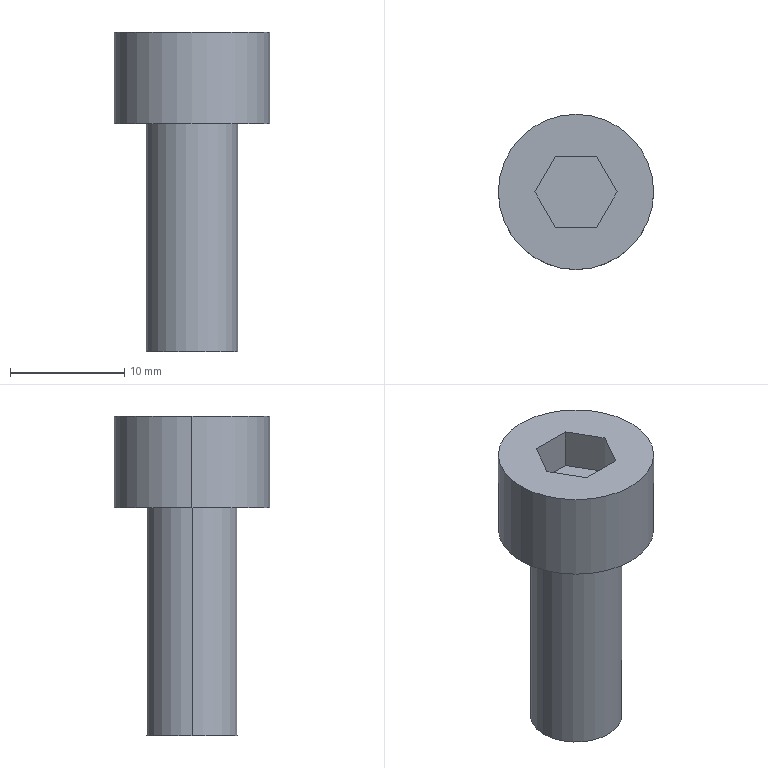Part | SolidWorks | features BaseBody 1 | 1 solid | 14 faces | box 13.6 x 13.6 x 28 mm | volume 2046 mm3 | plane 10 | cylinder 4 | commonest cylinder face diameters 8 x2 13.6 x2
STEP:
#1=CARTESIAN_POINT('',(4.,0.,-20.));
#2=VERTEX_POINT('',#1);
#3=CARTESIAN_POINT('',(-4.,0.,-20.));
#4=VERTEX_POINT('',#3);
#5=CARTESIAN_POINT('',(0.,0.,-20.));
#6=DIRECTION('',(0.,0.,1.));
#7=DIRECTION('',(1.,0.,0.));
#8=AXIS2_PLACEMENT_3D('',#5,#6,#7);
#9=CIRCLE('',#8,4.);
#10=EDGE_CURVE('',#2,#4,#9,.T.);
#11=ORIENTED_EDGE('',*,*,#10,.T.);
#12=CARTESIAN_POINT('',(-4.,0.,0.));
#13=VERTEX_POINT('',#12);
#14=CARTESIAN_POINT('',(-4.,0.,-20.));
#15=DIRECTION('',(0.,0.,1.));
#16=VECTOR('',#15,1000.);
#17=LINE('',#14,#16);
#18=EDGE_CURVE('',#4,#13,#17,.T.);
#19=ORIENTED_EDGE('',*,*,#18,.T.);
#20=CARTESIAN_POINT('',(4.,0.,0.));
#21=VERTEX_POINT('',#20);
#22=CARTESIAN_POINT('',(0.,0.,0.));
#23=DIRECTION('',(0.,0.,-1.));
#24=DIRECTION('',(1.,0.,0.));
#25=AXIS2_PLACEMENT_3D('',#22,#23,#24);
#26=CIRCLE('',#25,4.);
#27=EDGE_CURVE('',#13,#21,#26,.T.);
#28=ORIENTED_EDGE('',*,*,#27,.T.);
#29=CARTESIAN_POINT('',(4.,0.,-20.));
#30=DIRECTION('',(0.,0.,1.));
#31=VECTOR('',#30,1000.);
#32=LINE('',#29,#31);
#33=EDGE_CURVE('',#2,#21,#32,.T.);
#34=ORIENTED_EDGE('',*,*,#33,.F.);
#35=EDGE_LOOP('',(#11,#19,#28,#34));
#36=FACE_OUTER_BOUND('',#35,.T.);
#37=CARTESIAN_POINT('',(0.,0.,-20.));
#38=DIRECTION('',(0.,0.,1.));
#39=DIRECTION('',(1.,0.,0.));
#40=AXIS2_PLACEMENT_3D('',#37,#38,#39);
#41=CYLINDRICAL_SURFACE('',#40,4.);
#42=ADVANCED_FACE('',(#36),#41,.T.);
#43=CARTESIAN_POINT('',(6.8,0.,0.));
#44=VERTEX_POINT('',#43);
#45=CARTESIAN_POINT('',(-6.8,0.,0.));
#46=VERTEX_POINT('',#45);
#47=CARTESIAN_POINT('',(0.,0.,0.));
#48=DIRECTION('',(0.,0.,1.));
#49=DIRECTION('',(1.,0.,0.));
#50=AXIS2_PLACEMENT_3D('',#47,#48,#49);
#51=CIRCLE('',#50,6.8);
#52=EDGE_CURVE('',#44,#46,#51,.T.);
#53=ORIENTED_EDGE('',*,*,#52,.T.);
#54=CARTESIAN_POINT('',(-6.8,0.,8.));
#55=VERTEX_POINT('',#54);
#56=CARTESIAN_POINT('',(-6.8,0.,0.));
#57=DIRECTION('',(0.,0.,1.));
#58=VECTOR('',#57,1000.);
#59=LINE('',#56,#58);
#60=EDGE_CURVE('',#46,#55,#59,.T.);
#61=ORIENTED_EDGE('',*,*,#60,.T.);
#62=CARTESIAN_POINT('',(6.8,0.,8.));
#63=VERTEX_POINT('',#62);
#64=CARTESIAN_POINT('',(0.,0.,8.));
#65=DIRECTION('',(0.,0.,-1.));
#66=DIRECTION('',(1.,0.,0.));
#67=AXIS2_PLACEMENT_3D('',#64,#65,#66);
#68=CIRCLE('',#67,6.8);
#69=EDGE_CURVE('',#55,#63,#68,.T.);
#70=ORIENTED_EDGE('',*,*,#69,.T.);
#71=CARTESIAN_POINT('',(6.8,0.,0.));
#72=DIRECTION('',(0.,0.,1.));
#73=VECTOR('',#72,1000.);
#74=LINE('',#71,#73);
#75=EDGE_CURVE('',#44,#63,#74,.T.);
#76=ORIENTED_EDGE('',*,*,#75,.F.);
#77=EDGE_LOOP('',(#53,#61,#70,#76));
#78=FACE_OUTER_BOUND('',#77,.T.);
#79=CARTESIAN_POINT('',(0.,0.,0.));
#80=DIRECTION('',(0.,0.,1.));
#81=DIRECTION('',(1.,0.,0.));
#82=AXIS2_PLACEMENT_3D('',#79,#80,#81);
#83=CYLINDRICAL_SURFACE('',#82,6.8);
#84=ADVANCED_FACE('',(#78),#83,.T.);
#85=ORIENTED_EDGE('',*,*,#18,.F.);
#86=CARTESIAN_POINT('',(0.,0.,-20.));
#87=DIRECTION('',(0.,0.,1.));
#88=DIRECTION('',(1.,0.,0.));
#89=AXIS2_PLACEMENT_3D('',#86,#87,#88);
#90=CIRCLE('',#89,4.);
#91=EDGE_CURVE('',#4,#2,#90,.T.);
#92=ORIENTED_EDGE('',*,*,#91,.T.);
#93=ORIENTED_EDGE('',*,*,#33,.T.);
#94=CARTESIAN_POINT('',(0.,0.,0.));
#95=DIRECTION('',(0.,0.,-1.));
#96=DIRECTION('',(1.,0.,0.));
#97=AXIS2_PLACEMENT_3D('',#94,#95,#96);
#98=CIRCLE('',#97,4.);
#99=EDGE_CURVE('',#21,#13,#98,.T.);
#100=ORIENTED_EDGE('',*,*,#99,.T.);
#101=EDGE_LOOP('',(#85,#92,#93,#100));
#102=FACE_OUTER_BOUND('',#101,.T.);
#103=CARTESIAN_POINT('',(0.,0.,-20.));
#104=DIRECTION('',(0.,0.,1.));
#105=DIRECTION('',(1.,0.,0.));
#106=AXIS2_PLACEMENT_3D('',#103,#104,#105);
#107=CYLINDRICAL_SURFACE('',#106,4.);
#108=ADVANCED_FACE('',(#102),#107,.T.);
#109=ORIENTED_EDGE('',*,*,#10,.F.);
#110=ORIENTED_EDGE('',*,*,#91,.F.);
#111=EDGE_LOOP('',(#109,#110));
#112=FACE_OUTER_BOUND('',#111,.T.);
#113=CARTESIAN_POINT('',(0.,0.,-20.));
#114=DIRECTION('',(0.,0.,1.));
#115=DIRECTION('',(1.,0.,0.));
#116=AXIS2_PLACEMENT_3D('',#113,#114,#115);
#117=PLANE('',#116);
#118=ADVANCED_FACE('',(#112),#117,.F.);
#119=ORIENTED_EDGE('',*,*,#99,.F.);
#120=ORIENTED_EDGE('',*,*,#27,.F.);
#121=EDGE_LOOP('',(#119,#120));
#122=FACE_BOUND('',#121,.T.);
#123=ORIENTED_EDGE('',*,*,#52,.F.);
#124=CARTESIAN_POINT('',(0.,0.,0.));
#125=DIRECTION('',(0.,0.,1.));
#126=DIRECTION('',(1.,0.,0.));
#127=AXIS2_PLACEMENT_3D('',#124,#125,#126);
#128=CIRCLE('',#127,6.8);
#129=EDGE_CURVE('',#46,#44,#128,.T.);
#130=ORIENTED_EDGE('',*,*,#129,.F.);
#131=EDGE_LOOP('',(#123,#130));
#132=FACE_OUTER_BOUND('',#131,.T.);
#133=CARTESIAN_POINT('',(0.,0.,0.));
#134=DIRECTION('',(0.,0.,1.));
#135=DIRECTION('',(1.,0.,0.));
#136=AXIS2_PLACEMENT_3D('',#133,#134,#135);
#137=PLANE('',#136);
#138=ADVANCED_FACE('',(#122,#132),#137,.F.);
#139=ORIENTED_EDGE('',*,*,#60,.F.);
#140=ORIENTED_EDGE('',*,*,#129,.T.);
#141=ORIENTED_EDGE('',*,*,#75,.T.);
#142=CARTESIAN_POINT('',(0.,0.,8.));
#143=DIRECTION('',(0.,0.,-1.));
#144=DIRECTION('',(1.,0.,0.));
#145=AXIS2_PLACEMENT_3D('',#142,#143,#144);
#146=CIRCLE('',#145,6.8);
#147=EDGE_CURVE('',#63,#55,#146,.T.);
#148=ORIENTED_EDGE('',*,*,#147,.T.);
#149=EDGE_LOOP('',(#139,#140,#141,#148));
#150=FACE_OUTER_BOUND('',#149,.T.);
#151=CARTESIAN_POINT('',(0.,0.,0.));
#152=DIRECTION('',(0.,0.,1.));
#153=DIRECTION('',(1.,0.,0.));
#154=AXIS2_PLACEMENT_3D('',#151,#152,#153);
#155=CYLINDRICAL_SURFACE('',#154,6.8);
#156=ADVANCED_FACE('',(#150),#155,.T.);
#157=CARTESIAN_POINT('',(-1.8,-3.118,8.));
#158=VERTEX_POINT('',#157);
#159=CARTESIAN_POINT('',(-3.6,0.,8.));
#160=VERTEX_POINT('',#159);
#161=CARTESIAN_POINT('',(-1.8,-3.118,8.));
#162=DIRECTION('',(-0.5,0.866,0.));
#163=VECTOR('',#162,1000.);
#164=LINE('',#161,#163);
#165=EDGE_CURVE('',#158,#160,#164,.T.);
#166=ORIENTED_EDGE('',*,*,#165,.T.);
#167=CARTESIAN_POINT('',(-1.8,3.118,8.));
#168=VERTEX_POINT('',#167);
#169=CARTESIAN_POINT('',(-3.6,0.,8.));
#170=DIRECTION('',(0.5,0.866,0.));
#171=VECTOR('',#170,1000.);
#172=LINE('',#169,#171);
#173=EDGE_CURVE('',#160,#168,#172,.T.);
#174=ORIENTED_EDGE('',*,*,#173,.T.);
#175=CARTESIAN_POINT('',(1.8,3.118,8.));
#176=VERTEX_POINT('',#175);
#177=CARTESIAN_POINT('',(0.,3.118,8.));
#178=DIRECTION('',(1.,0.,0.));
#179=VECTOR('',#178,1000.);
#180=LINE('',#177,#179);
#181=EDGE_CURVE('',#168,#176,#180,.T.);
#182=ORIENTED_EDGE('',*,*,#181,.T.);
#183=CARTESIAN_POINT('',(3.6,0.,8.));
#184=VERTEX_POINT('',#183);
#185=CARTESIAN_POINT('',(1.8,3.118,8.));
#186=DIRECTION('',(0.5,-0.866,0.));
#187=VECTOR('',#186,1000.);
#188=LINE('',#185,#187);
#189=EDGE_CURVE('',#176,#184,#188,.T.);
#190=ORIENTED_EDGE('',*,*,#189,.T.);
#191=CARTESIAN_POINT('',(1.8,-3.118,8.));
#192=VERTEX_POINT('',#191);
#193=CARTESIAN_POINT('',(3.6,0.,8.));
#194=DIRECTION('',(-0.5,-0.866,0.));
#195=VECTOR('',#194,1000.);
#196=LINE('',#193,#195);
#197=EDGE_CURVE('',#184,#192,#196,.T.);
#198=ORIENTED_EDGE('',*,*,#197,.T.);
#199=CARTESIAN_POINT('',(0.,-3.118,8.));
#200=DIRECTION('',(-1.,0.,0.));
#201=VECTOR('',#200,1000.);
#202=LINE('',#199,#201);
#203=EDGE_CURVE('',#192,#158,#202,.T.);
#204=ORIENTED_EDGE('',*,*,#203,.T.);
#205=EDGE_LOOP('',(#166,#174,#182,#190,#198,#204));
#206=FACE_BOUND('',#205,.T.);
#207=ORIENTED_EDGE('',*,*,#147,.F.);
#208=ORIENTED_EDGE('',*,*,#69,.F.);
#209=EDGE_LOOP('',(#207,#208));
#210=FACE_OUTER_BOUND('',#209,.T.);
#211=CARTESIAN_POINT('',(0.,0.,8.));
#212=DIRECTION('',(0.,0.,1.));
#213=DIRECTION('',(1.,0.,0.));
#214=AXIS2_PLACEMENT_3D('',#211,#212,#213);
#215=PLANE('',#214);
#216=ADVANCED_FACE('',(#206,#210),#215,.T.);
#217=ORIENTED_EDGE('',*,*,#173,.F.);
#218=CARTESIAN_POINT('',(-3.6,0.,4.4));
#219=VERTEX_POINT('',#218);
#220=CARTESIAN_POINT('',(-3.6,0.,4.4));
#221=DIRECTION('',(0.,0.,-1.));
#222=VECTOR('',#221,1000.);
#223=LINE('',#220,#222);
#224=EDGE_CURVE('',#160,#219,#223,.T.);
#225=ORIENTED_EDGE('',*,*,#224,.T.);
#226=CARTESIAN_POINT('',(-1.8,3.118,4.4));
#227=VERTEX_POINT('',#226);
#228=CARTESIAN_POINT('',(-1.8,3.118,4.4));
#229=DIRECTION('',(0.5,0.866,0.));
#230=VECTOR('',#229,1000.);
#231=LINE('',#228,#230);
#232=EDGE_CURVE('',#219,#227,#231,.T.);
#233=ORIENTED_EDGE('',*,*,#232,.T.);
#234=CARTESIAN_POINT('',(-1.8,3.118,4.4));
#235=DIRECTION('',(0.,0.,1.));
#236=VECTOR('',#235,1000.);
#237=LINE('',#234,#236);
#238=EDGE_CURVE('',#227,#168,#237,.T.);
#239=ORIENTED_EDGE('',*,*,#238,.T.);
#240=EDGE_LOOP('',(#217,#225,#233,#239));
#241=FACE_OUTER_BOUND('',#240,.T.);
#242=CARTESIAN_POINT('',(-1.8,3.118,4.4));
#243=DIRECTION('',(0.866,-0.5,0.));
#244=DIRECTION('',(0.5,0.866,0.));
#245=AXIS2_PLACEMENT_3D('',#242,#243,#244);
#246=PLANE('',#245);
#247=ADVANCED_FACE('',(#241),#246,.T.);
#248=ORIENTED_EDGE('',*,*,#165,.F.);
#249=CARTESIAN_POINT('',(-1.8,-3.118,4.4));
#250=VERTEX_POINT('',#249);
#251=CARTESIAN_POINT('',(-1.8,-3.118,4.4));
#252=DIRECTION('',(0.,0.,-1.));
#253=VECTOR('',#252,1000.);
#254=LINE('',#251,#253);
#255=EDGE_CURVE('',#158,#250,#254,.T.);
#256=ORIENTED_EDGE('',*,*,#255,.T.);
#257=CARTESIAN_POINT('',(-3.6,0.,4.4));
#258=DIRECTION('',(-0.5,0.866,0.));
#259=VECTOR('',#258,1000.);
#260=LINE('',#257,#259);
#261=EDGE_CURVE('',#250,#219,#260,.T.);
#262=ORIENTED_EDGE('',*,*,#261,.T.);
#263=ORIENTED_EDGE('',*,*,#224,.F.);
#264=EDGE_LOOP('',(#248,#256,#262,#263));
#265=FACE_OUTER_BOUND('',#264,.T.);
#266=CARTESIAN_POINT('',(-3.6,0.,4.4));
#267=DIRECTION('',(0.866,0.5,0.));
#268=DIRECTION('',(-0.5,0.866,0.));
#269=AXIS2_PLACEMENT_3D('',#266,#267,#268);
#270=PLANE('',#269);
#271=ADVANCED_FACE('',(#265),#270,.T.);
#272=ORIENTED_EDGE('',*,*,#203,.F.);
#273=CARTESIAN_POINT('',(1.8,-3.118,4.4));
#274=VERTEX_POINT('',#273);
#275=CARTESIAN_POINT('',(1.8,-3.118,4.4));
#276=DIRECTION('',(0.,0.,-1.));
#277=VECTOR('',#276,1000.);
#278=LINE('',#275,#277);
#279=EDGE_CURVE('',#192,#274,#278,.T.);
#280=ORIENTED_EDGE('',*,*,#279,.T.);
#281=CARTESIAN_POINT('',(-1.8,-3.118,4.4));
#282=DIRECTION('',(-1.,0.,0.));
#283=VECTOR('',#282,1000.);
#284=LINE('',#281,#283);
#285=EDGE_CURVE('',#274,#250,#284,.T.);
#286=ORIENTED_EDGE('',*,*,#285,.T.);
#287=ORIENTED_EDGE('',*,*,#255,.F.);
#288=EDGE_LOOP('',(#272,#280,#286,#287));
#289=FACE_OUTER_BOUND('',#288,.T.);
#290=CARTESIAN_POINT('',(-1.8,-3.118,4.4));
#291=DIRECTION('',(0.,1.,0.));
#292=DIRECTION('',(-1.,0.,0.));
#293=AXIS2_PLACEMENT_3D('',#290,#291,#292);
#294=PLANE('',#293);
#295=ADVANCED_FACE('',(#289),#294,.T.);
#296=ORIENTED_EDGE('',*,*,#197,.F.);
#297=CARTESIAN_POINT('',(3.6,0.,4.4));
#298=VERTEX_POINT('',#297);
#299=CARTESIAN_POINT('',(3.6,0.,4.4));
#300=DIRECTION('',(0.,0.,-1.));
#301=VECTOR('',#300,1000.);
#302=LINE('',#299,#301);
#303=EDGE_CURVE('',#184,#298,#302,.T.);
#304=ORIENTED_EDGE('',*,*,#303,.T.);
#305=CARTESIAN_POINT('',(1.8,-3.118,4.4));
#306=DIRECTION('',(-0.5,-0.866,0.));
#307=VECTOR('',#306,1000.);
#308=LINE('',#305,#307);
#309=EDGE_CURVE('',#298,#274,#308,.T.);
#310=ORIENTED_EDGE('',*,*,#309,.T.);
#311=ORIENTED_EDGE('',*,*,#279,.F.);
#312=EDGE_LOOP('',(#296,#304,#310,#311));
#313=FACE_OUTER_BOUND('',#312,.T.);
#314=CARTESIAN_POINT('',(1.8,-3.118,4.4));
#315=DIRECTION('',(-0.866,0.5,0.));
#316=DIRECTION('',(-0.5,-0.866,0.));
#317=AXIS2_PLACEMENT_3D('',#314,#315,#316);
#318=PLANE('',#317);
#319=ADVANCED_FACE('',(#313),#318,.T.);
#320=ORIENTED_EDGE('',*,*,#189,.F.);
#321=CARTESIAN_POINT('',(1.8,3.118,4.4));
#322=VERTEX_POINT('',#321);
#323=CARTESIAN_POINT('',(1.8,3.118,4.4));
#324=DIRECTION('',(0.,0.,-1.));
#325=VECTOR('',#324,1000.);
#326=LINE('',#323,#325);
#327=EDGE_CURVE('',#176,#322,#326,.T.);
#328=ORIENTED_EDGE('',*,*,#327,.T.);
#329=CARTESIAN_POINT('',(3.6,0.,4.4));
#330=DIRECTION('',(0.5,-0.866,0.));
#331=VECTOR('',#330,1000.);
#332=LINE('',#329,#331);
#333=EDGE_CURVE('',#322,#298,#332,.T.);
#334=ORIENTED_EDGE('',*,*,#333,.T.);
#335=ORIENTED_EDGE('',*,*,#303,.F.);
#336=EDGE_LOOP('',(#320,#328,#334,#335));
#337=FACE_OUTER_BOUND('',#336,.T.);
#338=CARTESIAN_POINT('',(3.6,0.,4.4));
#339=DIRECTION('',(-0.866,-0.5,0.));
#340=DIRECTION('',(0.5,-0.866,0.));
#341=AXIS2_PLACEMENT_3D('',#338,#339,#340);
#342=PLANE('',#341);
#343=ADVANCED_FACE('',(#337),#342,.T.);
#344=ORIENTED_EDGE('',*,*,#181,.F.);
#345=ORIENTED_EDGE('',*,*,#238,.F.);
#346=CARTESIAN_POINT('',(1.8,3.118,4.4));
#347=DIRECTION('',(1.,0.,0.));
#348=VECTOR('',#347,1000.);
#349=LINE('',#346,#348);
#350=EDGE_CURVE('',#227,#322,#349,.T.);
#351=ORIENTED_EDGE('',*,*,#350,.T.);
#352=ORIENTED_EDGE('',*,*,#327,.F.);
#353=EDGE_LOOP('',(#344,#345,#351,#352));
#354=FACE_OUTER_BOUND('',#353,.T.);
#355=CARTESIAN_POINT('',(1.8,3.118,4.4));
#356=DIRECTION('',(0.,-1.,0.));
#357=DIRECTION('',(1.,0.,0.));
#358=AXIS2_PLACEMENT_3D('',#355,#356,#357);
#359=PLANE('',#358);
#360=ADVANCED_FACE('',(#354),#359,.T.);
#361=ORIENTED_EDGE('',*,*,#285,.F.);
#362=ORIENTED_EDGE('',*,*,#309,.F.);
#363=ORIENTED_EDGE('',*,*,#333,.F.);
#364=ORIENTED_EDGE('',*,*,#350,.F.);
#365=ORIENTED_EDGE('',*,*,#232,.F.);
#366=ORIENTED_EDGE('',*,*,#261,.F.);
#367=EDGE_LOOP('',(#361,#362,#363,#364,#365,#366));
#368=FACE_OUTER_BOUND('',#367,.T.);
#369=CARTESIAN_POINT('',(0.,0.,4.4));
#370=DIRECTION('',(0.,0.,1.));
#371=DIRECTION('',(1.,0.,0.));
#372=AXIS2_PLACEMENT_3D('',#369,#370,#371);
#373=PLANE('',#372);
#374=ADVANCED_FACE('',(#368),#373,.T.);
#375=CLOSED_SHELL('',(#42,#84,#108,#118,#138,#156,#216,#247,#271,#295,#319,#343,#360,#374));
#376=MANIFOLD_SOLID_BREP('',#375);
#377=CARTESIAN_POINT('',(0.,0.,0.));
#378=DIRECTION('',(0.,0.,1.));
#379=DIRECTION('',(1.,0.,0.));
#380=AXIS2_PLACEMENT_3D('',#377,#378,#379);
#381=(LENGTH_UNIT()NAMED_UNIT(*)SI_UNIT(.MILLI.,.METRE.));
#382=UNCERTAINTY_MEASURE_WITH_UNIT(LENGTH_MEASURE(0.00001),#381,'','');
#383=(NAMED_UNIT(*)PLANE_ANGLE_UNIT()SI_UNIT($,.RADIAN.));
#384=(NAMED_UNIT(*)SI_UNIT($,.STERADIAN.)SOLID_ANGLE_UNIT());
#385=(GEOMETRIC_REPRESENTATION_CONTEXT(3)GLOBAL_UNCERTAINTY_ASSIGNED_CONTEXT((#382))GLOBAL_UNIT_ASSIGNED_CONTEXT((#381,#383,#384))REPRESENTATION_CONTEXT('',''));
#386=ADVANCED_BREP_SHAPE_REPRESENTATION('',(#376,#380),#385);